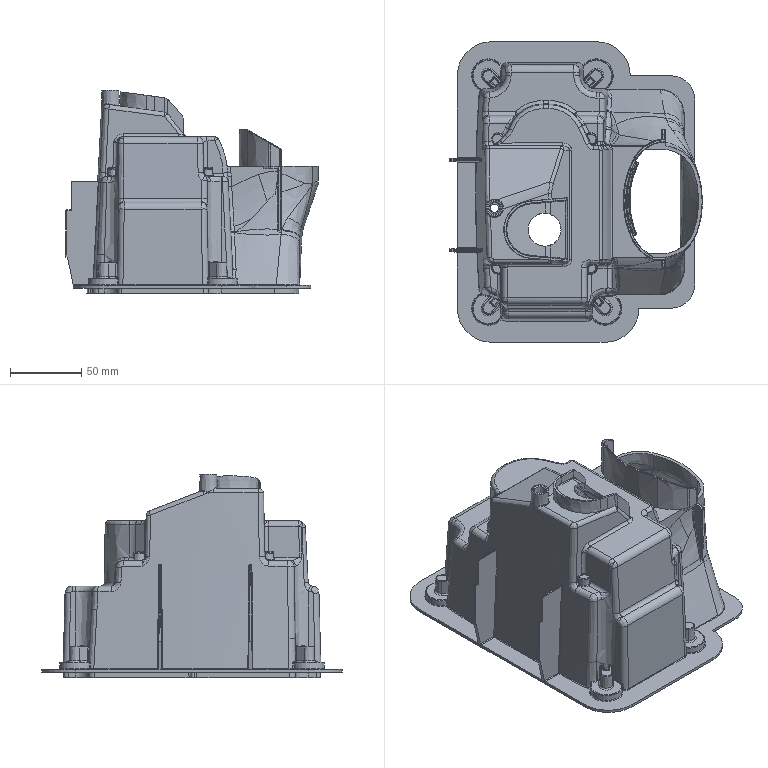Part | STEP file | solid 30 | 1 solid | 1785 faces | box 177.202 x 210.598 x 142.71 mm | volume 224641 mm3 | spline 812 | cylinder 389 | plane 261 | torus 151 | cone 99 | sphere 61 | other 12 | commonest cylinder face diameters 1.005 x126 0.502 x51 0.603 x46 3.216 x15 5.025 x15 2.01 x14